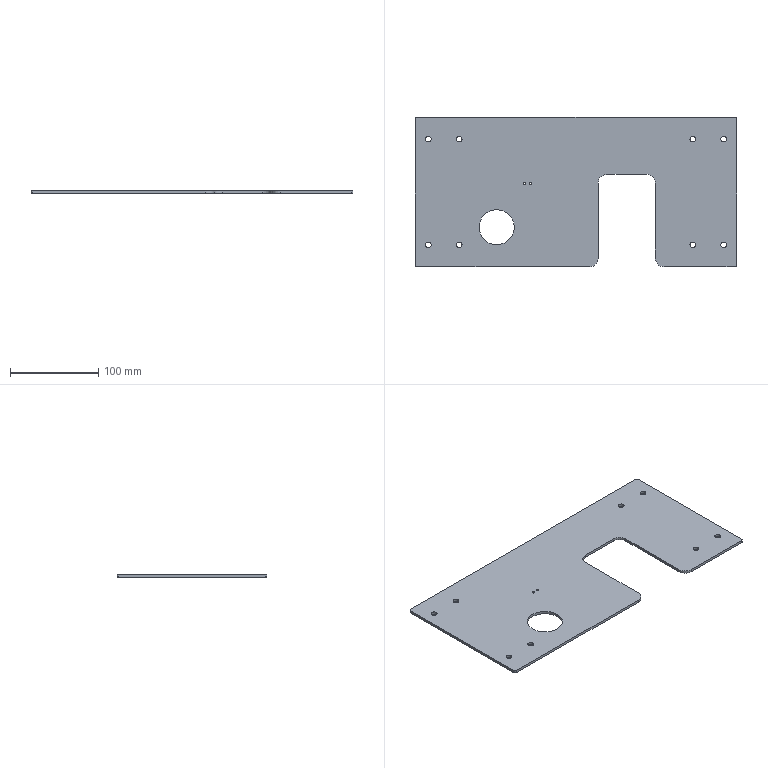Part | STEP file | 1 solid | 40 faces | box 365 x 170 x 3 mm | volume 161069 mm3 | cylinder 30 | plane 10 | commonest cylinder face diameters 6.5 x16 2.5 x4 4 x4 20 x4 40 x2